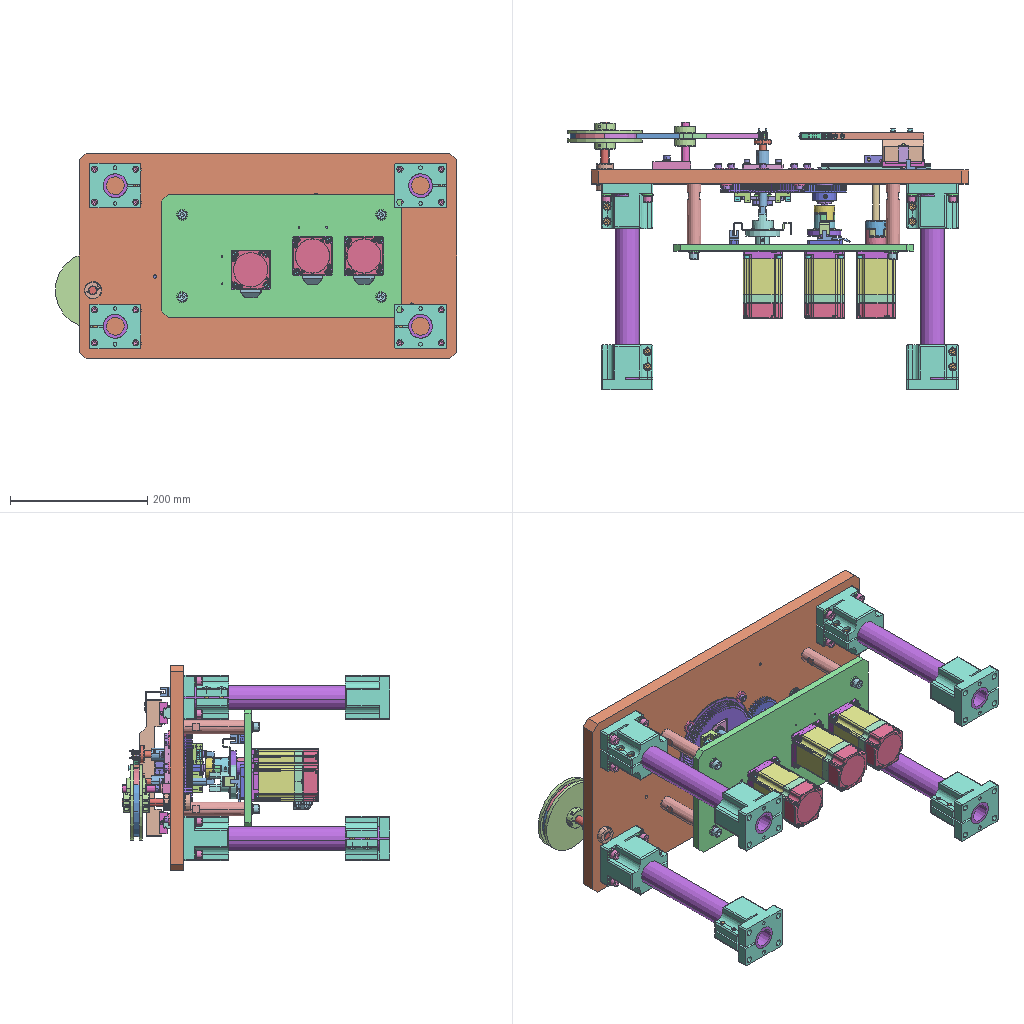Assembly | NX | 107 different items | 393 placed | box 585 x 390 x 300 mm
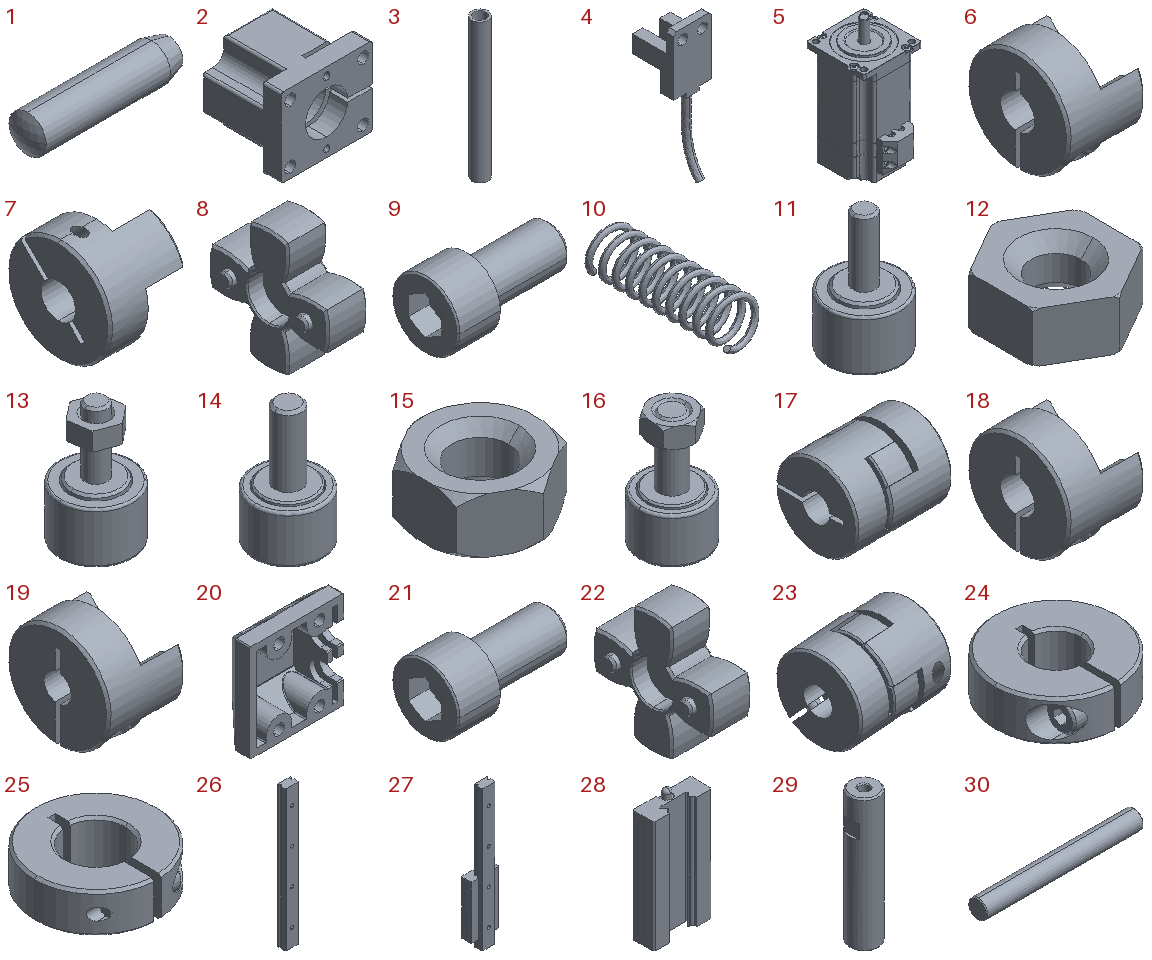Parts list (item | quantity | parent item | size | volume | features):
1 | x8 | - | 20 x 5 x 5 mm | 370.896 mm3 | features BREP 1
2 | x8 | - | 75 x 65 x 65 mm | 177792 mm3 | features BREP 1
3 | x4 | - | 35 x 35 x 300 mm | 129355 mm3 | features BREP 1
4 | x3 | - | 13.4 x 18.3 x 47.912 mm | 1659 mm3 | features BREP 1
5 | x3 | - | 57.15 x 69.65 x 119 mm | 168268 mm3 | features BREP 7
6 | x1 | in 17 | 22.5 x 30 x 29.981 mm | 7513 mm3 | features BREP 1
7 | x1 | in 17 | 22.5 x 30 x 30 mm | 7513 mm3 | features BREP 1
8 | x1 | in 17 | 13 x 30 x 30 mm | 3929 mm3 | features BREP 1
9 | x2 | in 17 | 12 x 6.4 x 6.4 mm | 210.2 mm3 | features BREP 1
10 | x2 | - | 4 x 12.497 x 4 mm | 21.567 mm3 | features BREP 1
11 | x2 | in 13 | 10 x 10 x 17 mm | 619.39 mm3 | features BREP 1
12 | x2 | in 13 | 5.5 x 6.351 x 2.5 mm | 50.092 mm3 | features BREP 1
13 | x2 | - | 10 x 10 x 17 mm | 669.482 mm3 | features BREP 2
14 | x1 | in 16 | 13 x 13 x 23 mm | 1465 mm3 | features BREP 1
15 | x1 | in 16 | 8 x 9.238 x 4 mm | 157.518 mm3 | features BREP 1
16 | x1 | - | 13 x 13 x 23 mm | 1623 mm3 | features BREP 2
17 | x1 | - | 35 x 30 x 30 mm | 19376 mm3 | features BREP 4
18 | x1 | in 23 | 22.5 x 30 x 29.981 mm | 7460 mm3 | features BREP 1
19 | x1 | in 23 | 22.5 x 30 x 29.981 mm | 7738 mm3 | features BREP 1
20 | x3 | in 5 | 29 x 12.5 x 30 mm | 3591 mm3 | features BREP 1
21 | x2 | in 23 | 12 x 6.4 x 6.4 mm | 210.2 mm3 | features BREP 1
22 | x1 | in 23 | 13 x 30 x 30 mm | 3929 mm3 | features BREP 1
23 | x1 | - | 36.579 x 31.222 x 30.842 mm | 19547 mm3 | features BREP 4
24 | x4 | - | 30 x 29.981 x 10 mm | 5567 mm3 | features BREP 1
25 | x2 | - | 25 x 24.977 x 9.5 mm | 2867 mm3 | features BREP 1
26 | x2 | in 27 | 15 x 9.5 x 160 mm | 20810 mm3 | features BREP 1
27 | x2 | - | 32 x 16 x 160 mm | 38851 mm3 | features BREP 2
28 | x2 | in 27 | 32 x 12 x 64.5 mm | 18041 mm3 | features BREP 1
29 | x4 | - | 20 x 20 x 93 mm | 27742 mm3 | features BREP 1
30 | x1 | - | 100 x 12 x 12 mm | 11301 mm3 | features BREP 1
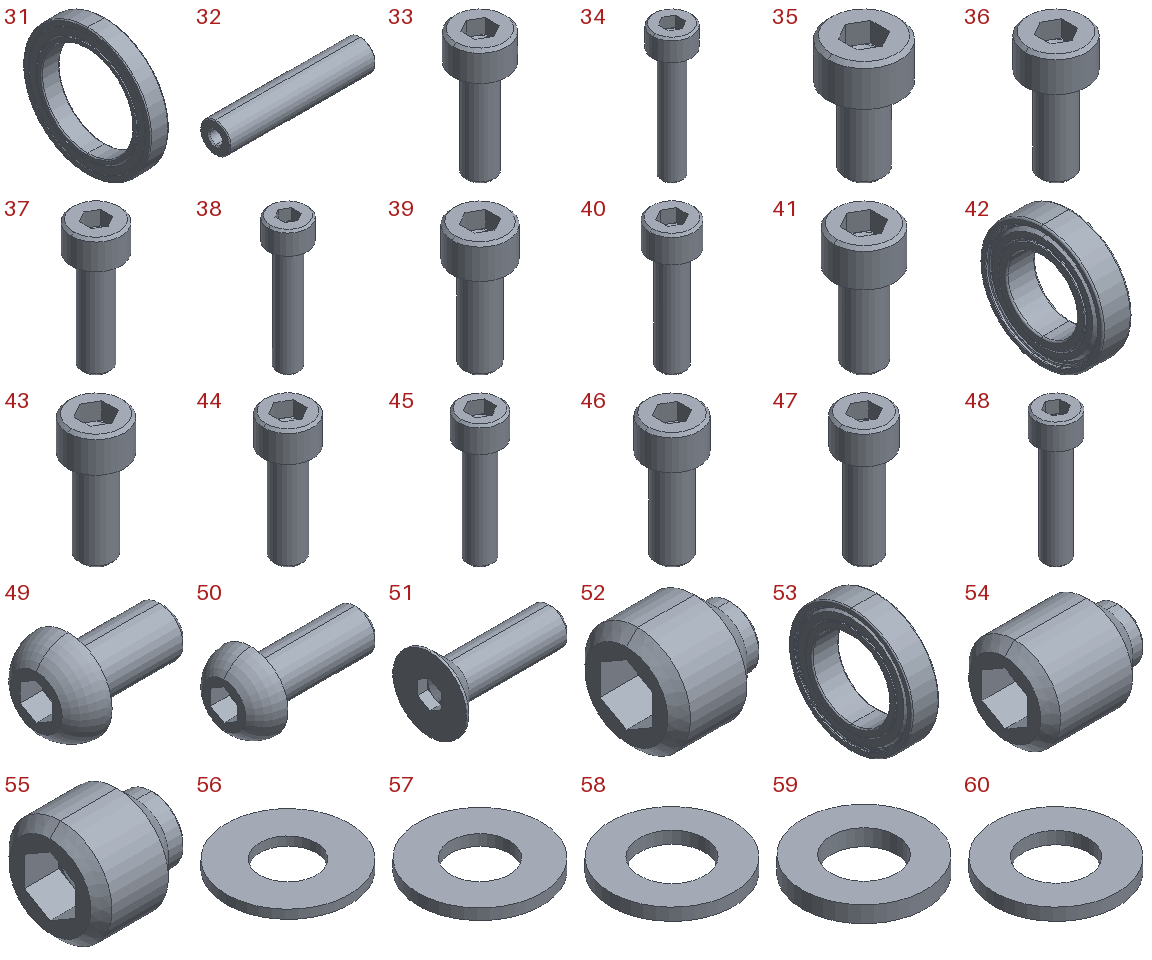31 | x1 | - | 20 x 140 x 140 mm | 112860 mm3 | features BREP 32
32 | x1 | - | 58 x 12 x 12 mm | 6309 mm3 | features BREP 1
33 | x12 | - | 5.5 x 5.5 x 13 mm | 131.617 mm3 | features BREP 1
34 | x12 | - | 5.5 x 5.5 x 19 mm | 174.028 mm3 | features BREP 1
35 | x4 | - | 5.5 x 5.5 x 9 mm | 103.342 mm3 | features BREP 1
36 | x8 | - | 5.5 x 5.5 x 11 mm | 117.48 mm3 | features BREP 1
37 | x12 | - | 7 x 7 x 18 mm | 309.86 mm3 | features BREP 1
38 | x2 | - | 7 x 7 x 24 mm | 385.258 mm3 | features BREP 1
39 | x1 | - | 8.5 x 8.5 x 19 mm | 515.039 mm3 | features BREP 1
40 | x4 | - | 8.5 x 8.5 x 25 mm | 632.849 mm3 | features BREP 1
41 | x11 | - | 10 x 10 x 20 mm | 785.579 mm3 | features BREP 1
42 | x6 | - | 5 x 21 x 21 mm | 897.771 mm3 | features BREP 1
43 | x1 | - | 10 x 10 x 22 mm | 842.128 mm3 | features BREP 1
44 | x16 | - | 10 x 10 x 26 mm | 955.225 mm3 | features BREP 1
45 | x1 | - | 10 x 10 x 31 mm | 1097 mm3 | features BREP 1
46 | x4 | - | 13 x 13 x 30 mm | 2011 mm3 | features BREP 1
47 | x4 | - | 13 x 13 x 33 mm | 2162 mm3 | features BREP 1
48 | x16 | - | 13 x 13 x 43 mm | 2665 mm3 | features BREP 1
49 | x8 | - | 8 x 5.5 x 5.5 mm | 74.567 mm3 | features BREP 1
50 | x6 | - | 10 x 5.5 x 5.5 mm | 88.704 mm3 | features BREP 1
51 | x2 | - | 10 x 6 x 6 mm | 85.103 mm3 | features BREP 1
52 | x4 | - | 4 x 4 x 4 mm | 34.482 mm3 | features BREP 1
53 | x2 | - | 7 x 32 x 32 mm | 2844 mm3 | features BREP 1
54 | x4 | - | 5 x 4 x 4 mm | 47.048 mm3 | features BREP 1
55 | x2 | - | 6 x 6 x 6 mm | 120.9 mm3 | features BREP 1
56 | x4 | - | 7 x 7 x 0.5 mm | 15.221 mm3 | features BREP 1
57 | x14 | - | 9 x 9 x 0.8 mm | 39.276 mm3 | features BREP 1
58 | x4 | - | 10 x 10 x 1 mm | 56.478 mm3 | features BREP 1
59 | x1 | - | 12 x 12 x 1.6 mm | 129.484 mm3 | features BREP 1
60 | x20 | - | 16 x 16 x 1.6 mm | 233.031 mm3 | features BREP 1
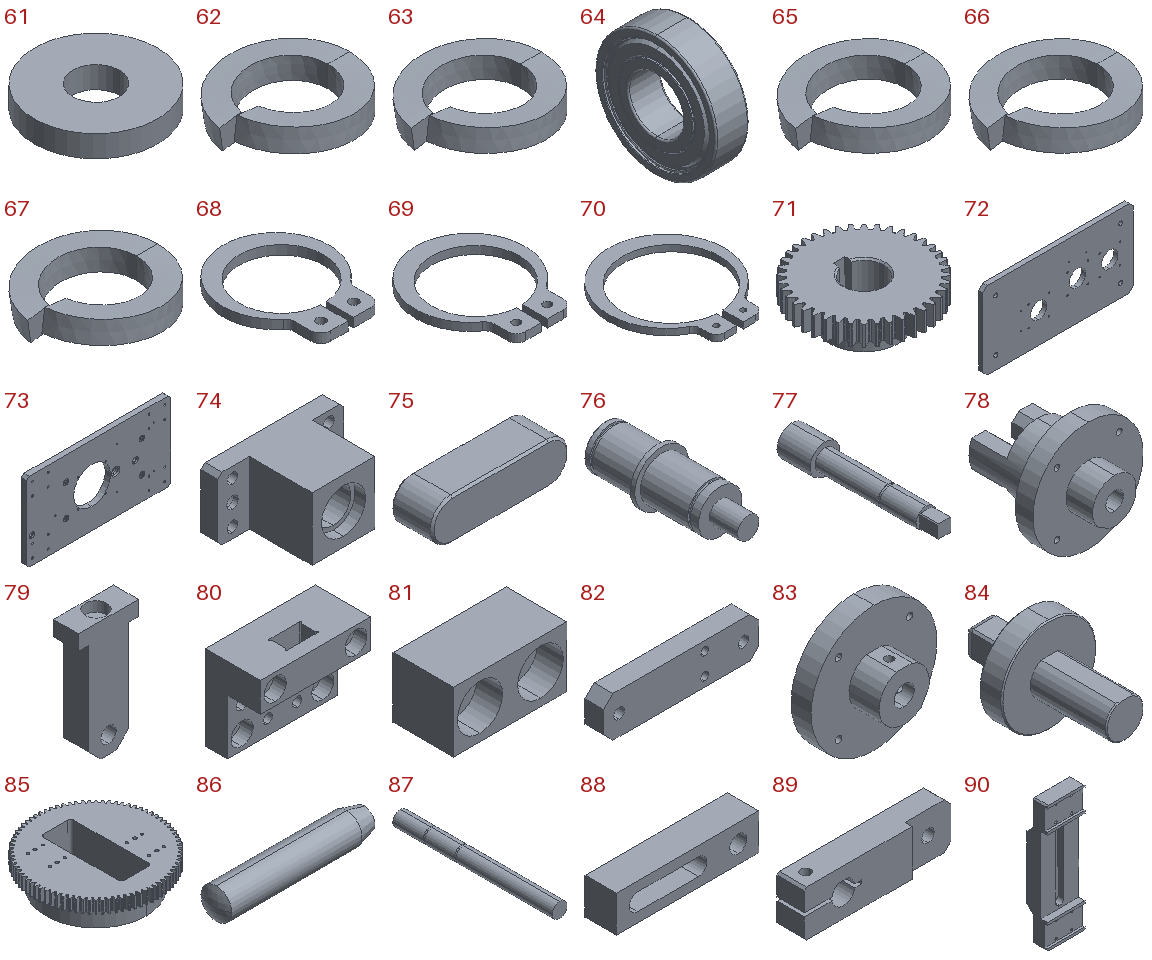61 | x11 | - | 17 x 17 x 3 mm | 584.43 mm3 | features BREP 1
62 | x14 | - | 6.827 x 6.867 x 2.131 mm | 24.116 mm3 | features BREP 1
63 | x4 | - | 8.227 x 8.278 x 2.523 mm | 39.802 mm3 | features BREP 1
64 | x2 | - | 6 x 22 x 22 mm | 1448 mm3 | features BREP 1
65 | x1 | - | 10.114 x 10.174 x 3.081 mm | 72.418 mm3 | features BREP 1
66 | x20 | - | 13.121 x 13.202 x 3.992 mm | 157.257 mm3 | features BREP 1
67 | x4 | - | 5.22 x 5.25 x 1.612 mm | 10.428 mm3 | features BREP 1
68 | x2 | - | 11.7 x 14.1 x 1 mm | 53.779 mm3 | features BREP 1
69 | x2 | - | 13.9 x 16.4 x 1 mm | 70.676 mm3 | features BREP 1
70 | x2 | - | 22.1 x 25.1 x 1.2 mm | 165.202 mm3 | features BREP 1
71 | x1 | - | 63 x 63 x 22 mm | 31779 mm3 | features BREP 1
72 | x1 | - | 350 x 10 x 180 mm | 587524 mm3 | features BREP 1
73 | x1 | - | 550 x 20 x 300 mm | 2934740 mm3 | features BREP 1
74 | x2 | - | 60 x 38 x 30 mm | 29884 mm3 | features BREP 1
75 | x1 | - | 20 x 6 x 6 mm | 669.486 mm3 | features BREP 1
76 | x1 | - | 25 x 66 x 25 mm | 17523 mm3 | features BREP 1
77 | x2 | - | 17.5 x 92 x 18 mm | 11638 mm3 | features BREP 1
78 | x1 | - | 50 x 51 x 50 mm | 32807 mm3 | features BREP 1
79 | x2 | - | 12 x 5 x 24 mm | 921.968 mm3 | features BREP 1
80 | x2 | - | 30 x 15 x 23 mm | 5187 mm3 | features BREP 1
81 | x2 | - | 15 x 8 x 8 mm | 660.349 mm3 | features BREP 1
82 | x2 | - | 50 x 6 x 13 mm | 3494 mm3 | features BREP 1
83 | x1 | - | 50 x 33 x 50 mm | 19638 mm3 | features BREP 1
84 | x2 | - | 25 x 38 x 25 mm | 5056 mm3 | features BREP 1
85 | x1 | - | 123 x 123 x 32 mm | 210252 mm3 | features BREP 1
86 | x4 | - | 15 x 3 x 3 mm | 100.309 mm3 | features BREP 1
87 | x1 | - | 10 x 108 x 10 mm | 8451 mm3 | features BREP 1
88 | x1 | - | 55 x 12 x 14 mm | 6152 mm3 | features BREP 1
89 | x1 | - | 67 x 12 x 20 mm | 12717 mm3 | features BREP 1
90 | x1 | - | 60 x 32 x 200 mm | 228373 mm3 | features BREP 1
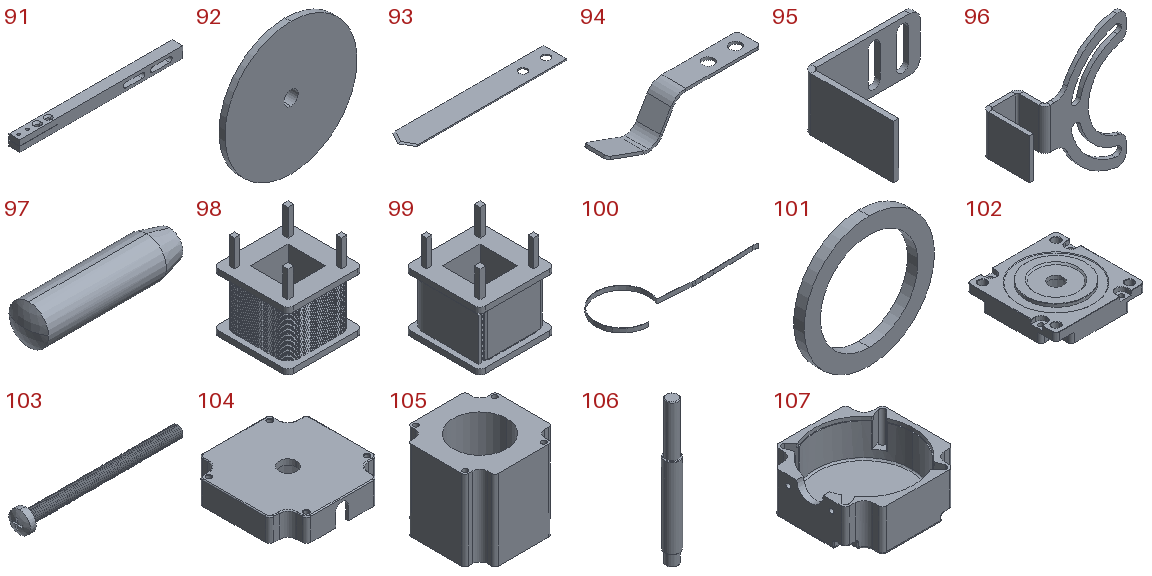91 | x1 | - | 150 x 10 x 10 mm | 12850 mm3 | features BREP 1
92 | x2 | - | 110 x 9 x 110 mm | 63935 mm3 | features BREP 1
93 | x1 | - | 68 x 10 x 0.5 mm | 320.283 mm3 | features BREP 1
94 | x2 | - | 45.274 x 7 x 10.8 mm | 268.431 mm3 | features BREP 1
95 | x1 | - | 31.5 x 25.5 x 15 mm | 1114 mm3 | features BREP 1
96 | x3 | - | 41.5 x 17.5 x 49.267 mm | 1595 mm3 | features BREP 1
97 | x4 | - | 15 x 4 x 4 mm | 174.937 mm3 | features BREP 1
98 | x1 | - | 14 x 14 x 16 mm | 814.621 mm3 | features BREP 46
99 | x1 | - | 14 x 14 x 16 mm | 921.369 mm3 | features BREP 46, LINKED_BODY 1
100 | x1 | - | 287.083 x 101 x 8 mm | 631.847 mm3 | features BREP 2, Delete Body 2, LINKED_FACE 2, SPLIT BODY 2, DATUM_PLANE 1
101 | x1 | - | 100 x 8 x 100 mm | 27489 mm3 | features BREP 1
102 | x3 | in 5 | 57.15 x 57.15 x 13.6 mm | 19483 mm3 | features BREP 1
103 | x12 | in 5 | 42.388 x 5.6 x 5.6 mm | 256.849 mm3 | features BREP 1
104 | x3 | in 5 | 57.15 x 57.15 x 13.4 mm | 17419 mm3 | features BREP 1
105 | x3 | in 5 | 57.15 x 57.15 x 52.6 mm | 100652 mm3 | features BREP 1
106 | x3 | in 5 | 10 x 10 x 95.8 mm | 6313 mm3 | features BREP 1
107 | x3 | in 5 | 57.15 x 57.15 x 22 mm | 19756 mm3 | features BREP 1